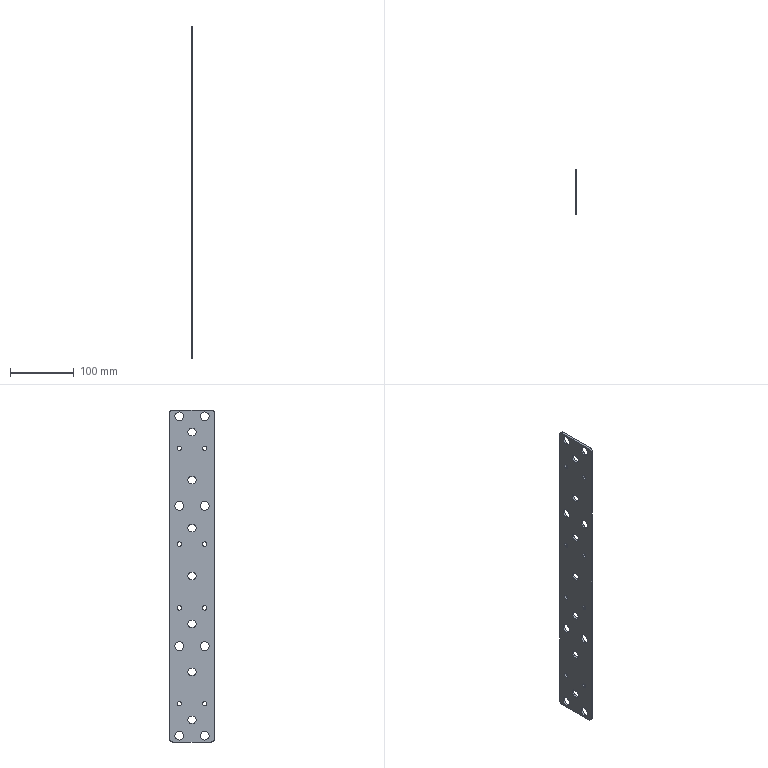Part | STEP file | 1 solid | 70 faces | box 3 x 70 x 520 mm | volume 101913 mm3 | cylinder 50 | plane 20 | commonest cylinder face diameters 7 x16 14 x16 13 x14 10 x4